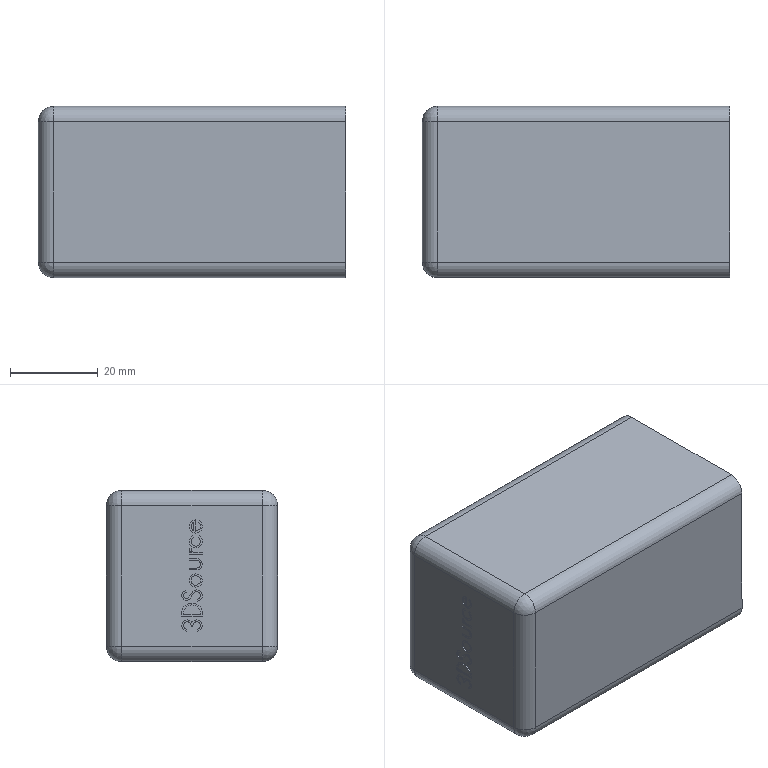Part | NX | features BREP 1 | 1 solid | 93 faces | box 70 x 39 x 39 mm | volume 105347 mm3 | plane 50 | cylinder 39 | sphere 4 | commonest cylinder face diameters 7 x8 1.712 x7 2.14 x6 2.55 x4 2.996 x4 2.568 x3